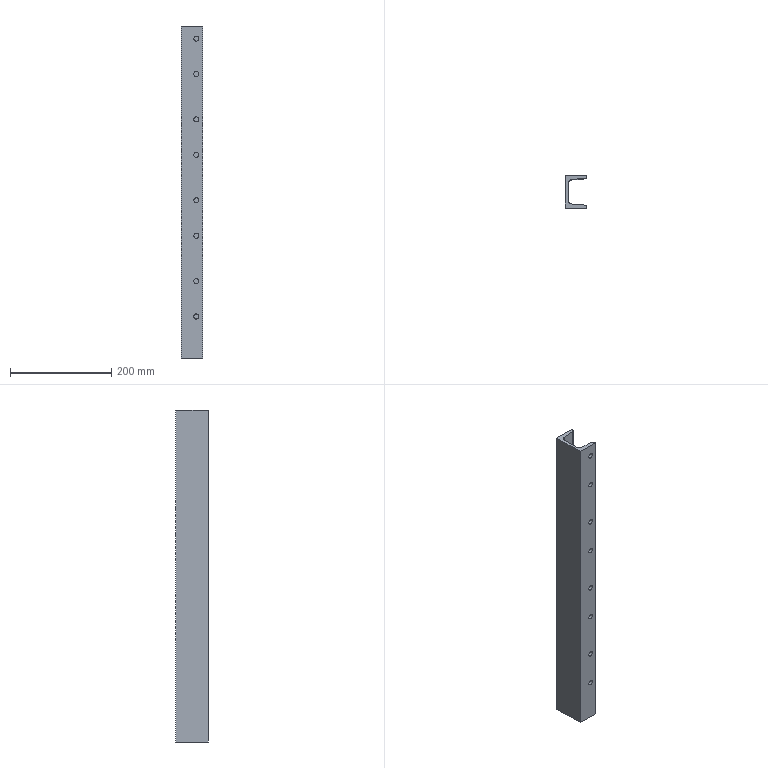Part | STEP file | DIN 1026-1 U 65 1785352674799 | 1 solid | 22 faces | box 42 x 65 x 657.157 mm | volume 589289 mm3 | cylinder 12 | plane 10 | commonest cylinder face diameters 10 x8 8 x2 15 x2
STEP:
#1=CARTESIAN_POINT('',(12.402,-24.312,657.157));
#2=VERTEX_POINT('',#1);
#3=CARTESIAN_POINT('',(38.319,-26.386,657.157));
#4=VERTEX_POINT('',#3);
#5=CARTESIAN_POINT('',(15.707,-24.577,657.157));
#6=DIRECTION('',(0.9968,-0.07975,0.));
#7=VECTOR('',#6,10.);
#8=LINE('',#5,#7);
#9=EDGE_CURVE('',#2,#4,#8,.T.);
#10=ORIENTED_EDGE('',*,*,#9,.F.);
#11=CARTESIAN_POINT('',(5.5,-16.836,657.157));
#12=VERTEX_POINT('',#11);
#13=CARTESIAN_POINT('',(13.,-16.836,657.157));
#14=DIRECTION('',(0.,0.,1.));
#15=DIRECTION('',(-1.,0.,0.));
#16=AXIS2_PLACEMENT_3D('',#13,#14,#15);
#17=CIRCLE('',#16,7.5);
#18=EDGE_CURVE('',#12,#2,#17,.T.);
#19=ORIENTED_EDGE('',*,*,#18,.F.);
#20=CARTESIAN_POINT('',(5.5,16.836,657.157));
#21=VERTEX_POINT('',#20);
#22=CARTESIAN_POINT('',(5.5,0.,657.157));
#23=DIRECTION('',(0.,-1.,0.));
#24=VECTOR('',#23,10.);
#25=LINE('',#22,#24);
#26=EDGE_CURVE('',#21,#12,#25,.T.);
#27=ORIENTED_EDGE('',*,*,#26,.F.);
#28=CARTESIAN_POINT('',(12.402,24.312,657.157));
#29=VERTEX_POINT('',#28);
#30=CARTESIAN_POINT('',(13.,16.836,657.157));
#31=DIRECTION('',(0.,0.,1.));
#32=DIRECTION('',(-0.07975,0.9968,0.));
#33=AXIS2_PLACEMENT_3D('',#30,#31,#32);
#34=CIRCLE('',#33,7.5);
#35=EDGE_CURVE('',#29,#21,#34,.T.);
#36=ORIENTED_EDGE('',*,*,#35,.F.);
#37=CARTESIAN_POINT('',(38.319,26.386,657.157));
#38=VERTEX_POINT('',#37);
#39=CARTESIAN_POINT('',(28.666,25.613,657.157));
#40=DIRECTION('',(-0.9968,-0.07975,0.));
#41=VECTOR('',#40,10.);
#42=LINE('',#39,#41);
#43=EDGE_CURVE('',#38,#29,#42,.T.);
#44=ORIENTED_EDGE('',*,*,#43,.F.);
#45=CARTESIAN_POINT('',(42.,30.373,657.157));
#46=VERTEX_POINT('',#45);
#47=CARTESIAN_POINT('',(38.,30.373,657.157));
#48=DIRECTION('',(0.,0.,-1.));
#49=DIRECTION('',(-0.07975,0.9968,0.));
#50=AXIS2_PLACEMENT_3D('',#47,#48,#49);
#51=CIRCLE('',#50,4.);
#52=EDGE_CURVE('',#46,#38,#51,.T.);
#53=ORIENTED_EDGE('',*,*,#52,.F.);
#54=CARTESIAN_POINT('',(42.,32.5,657.157));
#55=VERTEX_POINT('',#54);
#56=CARTESIAN_POINT('',(42.,16.25,657.157));
#57=DIRECTION('',(0.,-1.,0.));
#58=VECTOR('',#57,10.);
#59=LINE('',#56,#58);
#60=EDGE_CURVE('',#55,#46,#59,.T.);
#61=ORIENTED_EDGE('',*,*,#60,.F.);
#62=CARTESIAN_POINT('',(0.,32.5,657.157));
#63=VERTEX_POINT('',#62);
#64=CARTESIAN_POINT('',(10.5,32.5,657.157));
#65=DIRECTION('',(1.,0.,0.));
#66=VECTOR('',#65,10.);
#67=LINE('',#64,#66);
#68=EDGE_CURVE('',#63,#55,#67,.T.);
#69=ORIENTED_EDGE('',*,*,#68,.F.);
#70=CARTESIAN_POINT('',(0.,-32.5,657.157));
#71=VERTEX_POINT('',#70);
#72=CARTESIAN_POINT('',(0.,0.,657.157));
#73=DIRECTION('',(0.,1.,0.));
#74=VECTOR('',#73,10.);
#75=LINE('',#72,#74);
#76=EDGE_CURVE('',#71,#63,#75,.T.);
#77=ORIENTED_EDGE('',*,*,#76,.F.);
#78=CARTESIAN_POINT('',(42.,-32.5,657.157));
#79=VERTEX_POINT('',#78);
#80=CARTESIAN_POINT('',(31.5,-32.5,657.157));
#81=DIRECTION('',(-1.,0.,0.));
#82=VECTOR('',#81,10.);
#83=LINE('',#80,#82);
#84=EDGE_CURVE('',#79,#71,#83,.T.);
#85=ORIENTED_EDGE('',*,*,#84,.F.);
#86=CARTESIAN_POINT('',(42.,-30.373,657.157));
#87=VERTEX_POINT('',#86);
#88=CARTESIAN_POINT('',(42.,-15.186,657.157));
#89=DIRECTION('',(0.,-1.,0.));
#90=VECTOR('',#89,10.);
#91=LINE('',#88,#90);
#92=EDGE_CURVE('',#87,#79,#91,.T.);
#93=ORIENTED_EDGE('',*,*,#92,.F.);
#94=CARTESIAN_POINT('',(38.,-30.373,657.157));
#95=DIRECTION('',(0.,0.,-1.));
#96=DIRECTION('',(-1.,0.,0.));
#97=AXIS2_PLACEMENT_3D('',#94,#95,#96);
#98=CIRCLE('',#97,4.);
#99=EDGE_CURVE('',#4,#87,#98,.T.);
#100=ORIENTED_EDGE('',*,*,#99,.F.);
#101=EDGE_LOOP('',(#10,#19,#27,#36,#44,#53,#61,#69,#77,#85,#93,#100));
#102=FACE_OUTER_BOUND('',#101,.T.);
#103=CARTESIAN_POINT('',(21.,0.,657.157));
#104=DIRECTION('',(0.,0.,1.));
#105=DIRECTION('',(-1.,0.,0.));
#106=AXIS2_PLACEMENT_3D('',#103,#104,#105);
#107=PLANE('',#106);
#108=ADVANCED_FACE('',(#102),#107,.T.);
#109=ORIENTED_EDGE('',*,*,#52,.T.);
#110=CARTESIAN_POINT('',(38.319,26.386,0.));
#111=VERTEX_POINT('',#110);
#112=CARTESIAN_POINT('',(38.319,26.386,0.));
#113=DIRECTION('',(0.,0.,1.));
#114=VECTOR('',#113,10.);
#115=LINE('',#112,#114);
#116=EDGE_CURVE('',#111,#38,#115,.T.);
#117=ORIENTED_EDGE('',*,*,#116,.F.);
#118=CARTESIAN_POINT('',(42.,30.373,0.));
#119=VERTEX_POINT('',#118);
#120=CARTESIAN_POINT('',(38.,30.373,0.));
#121=DIRECTION('',(0.,0.,-1.));
#122=DIRECTION('',(-0.07975,0.9968,0.));
#123=AXIS2_PLACEMENT_3D('',#120,#121,#122);
#124=CIRCLE('',#123,4.);
#125=EDGE_CURVE('',#119,#111,#124,.T.);
#126=ORIENTED_EDGE('',*,*,#125,.F.);
#127=CARTESIAN_POINT('',(42.,30.373,0.));
#128=DIRECTION('',(0.,0.,1.));
#129=VECTOR('',#128,10.);
#130=LINE('',#127,#129);
#131=EDGE_CURVE('',#119,#46,#130,.T.);
#132=ORIENTED_EDGE('',*,*,#131,.T.);
#133=EDGE_LOOP('',(#109,#117,#126,#132));
#134=FACE_OUTER_BOUND('',#133,.T.);
#135=CARTESIAN_POINT('',(38.,30.373,0.));
#136=DIRECTION('',(0.,0.,1.));
#137=DIRECTION('',(-0.07975,0.9968,0.));
#138=AXIS2_PLACEMENT_3D('',#135,#136,#137);
#139=CYLINDRICAL_SURFACE('',#138,4.);
#140=ADVANCED_FACE('',(#134),#139,.T.);
#141=ORIENTED_EDGE('',*,*,#43,.T.);
#142=CARTESIAN_POINT('',(12.402,24.312,0.));
#143=VERTEX_POINT('',#142);
#144=CARTESIAN_POINT('',(12.402,24.312,0.));
#145=DIRECTION('',(0.,0.,1.));
#146=VECTOR('',#145,10.);
#147=LINE('',#144,#146);
#148=EDGE_CURVE('',#143,#29,#147,.T.);
#149=ORIENTED_EDGE('',*,*,#148,.F.);
#150=CARTESIAN_POINT('',(28.666,25.613,0.));
#151=DIRECTION('',(-0.9968,-0.07975,0.));
#152=VECTOR('',#151,10.);
#153=LINE('',#150,#152);
#154=EDGE_CURVE('',#111,#143,#153,.T.);
#155=ORIENTED_EDGE('',*,*,#154,.F.);
#156=ORIENTED_EDGE('',*,*,#116,.T.);
#157=EDGE_LOOP('',(#141,#149,#155,#156));
#158=FACE_OUTER_BOUND('',#157,.T.);
#159=CARTESIAN_POINT('',(38.319,26.386,0.));
#160=DIRECTION('',(0.07975,-0.9968,0.));
#161=DIRECTION('',(0.,0.,-1.));
#162=AXIS2_PLACEMENT_3D('',#159,#160,#161);
#163=PLANE('',#162);
#164=ADVANCED_FACE('',(#158),#163,.T.);
#165=ORIENTED_EDGE('',*,*,#35,.T.);
#166=CARTESIAN_POINT('',(5.5,16.836,0.));
#167=VERTEX_POINT('',#166);
#168=CARTESIAN_POINT('',(5.5,16.836,0.));
#169=DIRECTION('',(0.,0.,1.));
#170=VECTOR('',#169,10.);
#171=LINE('',#168,#170);
#172=EDGE_CURVE('',#167,#21,#171,.T.);
#173=ORIENTED_EDGE('',*,*,#172,.F.);
#174=CARTESIAN_POINT('',(13.,16.836,0.));
#175=DIRECTION('',(0.,0.,1.));
#176=DIRECTION('',(-0.07975,0.9968,0.));
#177=AXIS2_PLACEMENT_3D('',#174,#175,#176);
#178=CIRCLE('',#177,7.5);
#179=EDGE_CURVE('',#143,#167,#178,.T.);
#180=ORIENTED_EDGE('',*,*,#179,.F.);
#181=ORIENTED_EDGE('',*,*,#148,.T.);
#182=EDGE_LOOP('',(#165,#173,#180,#181));
#183=FACE_OUTER_BOUND('',#182,.T.);
#184=CARTESIAN_POINT('',(13.,16.836,0.));
#185=DIRECTION('',(0.,0.,1.));
#186=DIRECTION('',(-0.07975,0.9968,0.));
#187=AXIS2_PLACEMENT_3D('',#184,#185,#186);
#188=CYLINDRICAL_SURFACE('',#187,7.5);
#189=ADVANCED_FACE('',(#183),#188,.F.);
#190=ORIENTED_EDGE('',*,*,#26,.T.);
#191=CARTESIAN_POINT('',(5.5,-16.836,0.));
#192=VERTEX_POINT('',#191);
#193=CARTESIAN_POINT('',(5.5,-16.836,0.));
#194=DIRECTION('',(0.,0.,1.));
#195=VECTOR('',#194,10.);
#196=LINE('',#193,#195);
#197=EDGE_CURVE('',#192,#12,#196,.T.);
#198=ORIENTED_EDGE('',*,*,#197,.F.);
#199=CARTESIAN_POINT('',(5.5,0.,0.));
#200=DIRECTION('',(0.,-1.,0.));
#201=VECTOR('',#200,10.);
#202=LINE('',#199,#201);
#203=EDGE_CURVE('',#167,#192,#202,.T.);
#204=ORIENTED_EDGE('',*,*,#203,.F.);
#205=ORIENTED_EDGE('',*,*,#172,.T.);
#206=EDGE_LOOP('',(#190,#198,#204,#205));
#207=FACE_OUTER_BOUND('',#206,.T.);
#208=CARTESIAN_POINT('',(5.5,0.,0.));
#209=DIRECTION('',(1.,0.,0.));
#210=DIRECTION('',(0.,0.,-1.));
#211=AXIS2_PLACEMENT_3D('',#208,#209,#210);
#212=PLANE('',#211);
#213=ADVANCED_FACE('',(#207),#212,.T.);
#214=ORIENTED_EDGE('',*,*,#18,.T.);
#215=CARTESIAN_POINT('',(12.402,-24.312,0.));
#216=VERTEX_POINT('',#215);
#217=CARTESIAN_POINT('',(12.402,-24.312,0.));
#218=DIRECTION('',(0.,0.,1.));
#219=VECTOR('',#218,10.);
#220=LINE('',#217,#219);
#221=EDGE_CURVE('',#216,#2,#220,.T.);
#222=ORIENTED_EDGE('',*,*,#221,.F.);
#223=CARTESIAN_POINT('',(13.,-16.836,0.));
#224=DIRECTION('',(0.,0.,1.));
#225=DIRECTION('',(-1.,0.,0.));
#226=AXIS2_PLACEMENT_3D('',#223,#224,#225);
#227=CIRCLE('',#226,7.5);
#228=EDGE_CURVE('',#192,#216,#227,.T.);
#229=ORIENTED_EDGE('',*,*,#228,.F.);
#230=ORIENTED_EDGE('',*,*,#197,.T.);
#231=EDGE_LOOP('',(#214,#222,#229,#230));
#232=FACE_OUTER_BOUND('',#231,.T.);
#233=CARTESIAN_POINT('',(13.,-16.836,0.));
#234=DIRECTION('',(0.,0.,1.));
#235=DIRECTION('',(-1.,0.,0.));
#236=AXIS2_PLACEMENT_3D('',#233,#234,#235);
#237=CYLINDRICAL_SURFACE('',#236,7.5);
#238=ADVANCED_FACE('',(#232),#237,.F.);
#239=ORIENTED_EDGE('',*,*,#9,.T.);
#240=CARTESIAN_POINT('',(38.319,-26.386,0.));
#241=VERTEX_POINT('',#240);
#242=CARTESIAN_POINT('',(38.319,-26.386,0.));
#243=DIRECTION('',(0.,0.,1.));
#244=VECTOR('',#243,10.);
#245=LINE('',#242,#244);
#246=EDGE_CURVE('',#241,#4,#245,.T.);
#247=ORIENTED_EDGE('',*,*,#246,.F.);
#248=CARTESIAN_POINT('',(15.707,-24.577,0.));
#249=DIRECTION('',(0.9968,-0.07975,0.));
#250=VECTOR('',#249,10.);
#251=LINE('',#248,#250);
#252=EDGE_CURVE('',#216,#241,#251,.T.);
#253=ORIENTED_EDGE('',*,*,#252,.F.);
#254=ORIENTED_EDGE('',*,*,#221,.T.);
#255=EDGE_LOOP('',(#239,#247,#253,#254));
#256=FACE_OUTER_BOUND('',#255,.T.);
#257=CARTESIAN_POINT('',(34.5,-26.08,632.157));
#258=VERTEX_POINT('',#257);
#259=CARTESIAN_POINT('',(29.5,-25.68,632.157));
#260=DIRECTION('',(-0.07975,-0.9968,0.));
#261=DIRECTION('',(-0.9968,0.07975,0.));
#262=AXIS2_PLACEMENT_3D('',#259,#260,#261);
#263=ELLIPSE('',#262,5.016,5.);
#264=EDGE_CURVE('',#258,#258,#263,.T.);
#265=ORIENTED_EDGE('',*,*,#264,.T.);
#266=EDGE_LOOP('',(#265));
#267=FACE_BOUND('',#266,.T.);
#268=CARTESIAN_POINT('',(34.5,-26.08,562.157));
#269=VERTEX_POINT('',#268);
#270=CARTESIAN_POINT('',(29.5,-25.68,562.157));
#271=DIRECTION('',(-0.07975,-0.9968,0.));
#272=DIRECTION('',(-0.9968,0.07975,0.));
#273=AXIS2_PLACEMENT_3D('',#270,#271,#272);
#274=ELLIPSE('',#273,5.016,5.);
#275=EDGE_CURVE('',#269,#269,#274,.T.);
#276=ORIENTED_EDGE('',*,*,#275,.T.);
#277=EDGE_LOOP('',(#276));
#278=FACE_BOUND('',#277,.T.);
#279=CARTESIAN_POINT('',(34.5,-26.08,472.157));
#280=VERTEX_POINT('',#279);
#281=CARTESIAN_POINT('',(29.5,-25.68,472.157));
#282=DIRECTION('',(-0.07975,-0.9968,0.));
#283=DIRECTION('',(-0.9968,0.07975,0.));
#284=AXIS2_PLACEMENT_3D('',#281,#282,#283);
#285=ELLIPSE('',#284,5.016,5.);
#286=EDGE_CURVE('',#280,#280,#285,.T.);
#287=ORIENTED_EDGE('',*,*,#286,.T.);
#288=EDGE_LOOP('',(#287));
#289=FACE_BOUND('',#288,.T.);
#290=CARTESIAN_POINT('',(34.5,-26.08,402.157));
#291=VERTEX_POINT('',#290);
#292=CARTESIAN_POINT('',(29.5,-25.68,402.157));
#293=DIRECTION('',(-0.07975,-0.9968,0.));
#294=DIRECTION('',(-0.9968,0.07975,0.));
#295=AXIS2_PLACEMENT_3D('',#292,#293,#294);
#296=ELLIPSE('',#295,5.016,5.);
#297=EDGE_CURVE('',#291,#291,#296,.T.);
#298=ORIENTED_EDGE('',*,*,#297,.T.);
#299=EDGE_LOOP('',(#298));
#300=FACE_BOUND('',#299,.T.);
#301=CARTESIAN_POINT('',(34.5,-26.08,312.157));
#302=VERTEX_POINT('',#301);
#303=CARTESIAN_POINT('',(29.5,-25.68,312.157));
#304=DIRECTION('',(-0.07975,-0.9968,0.));
#305=DIRECTION('',(-0.9968,0.07975,0.));
#306=AXIS2_PLACEMENT_3D('',#303,#304,#305);
#307=ELLIPSE('',#306,5.016,5.);
#308=EDGE_CURVE('',#302,#302,#307,.T.);
#309=ORIENTED_EDGE('',*,*,#308,.T.);
#310=EDGE_LOOP('',(#309));
#311=FACE_BOUND('',#310,.T.);
#312=CARTESIAN_POINT('',(34.5,-26.08,242.157));
#313=VERTEX_POINT('',#312);
#314=CARTESIAN_POINT('',(29.5,-25.68,242.157));
#315=DIRECTION('',(-0.07975,-0.9968,0.));
#316=DIRECTION('',(-0.9968,0.07975,0.));
#317=AXIS2_PLACEMENT_3D('',#314,#315,#316);
#318=ELLIPSE('',#317,5.016,5.);
#319=EDGE_CURVE('',#313,#313,#318,.T.);
#320=ORIENTED_EDGE('',*,*,#319,.T.);
#321=EDGE_LOOP('',(#320));
#322=FACE_BOUND('',#321,.T.);
#323=CARTESIAN_POINT('',(34.5,-26.08,152.157));
#324=VERTEX_POINT('',#323);
#325=CARTESIAN_POINT('',(29.5,-25.68,152.157));
#326=DIRECTION('',(-0.07975,-0.9968,0.));
#327=DIRECTION('',(-0.9968,0.07975,0.));
#328=AXIS2_PLACEMENT_3D('',#325,#326,#327);
#329=ELLIPSE('',#328,5.016,5.);
#330=EDGE_CURVE('',#324,#324,#329,.T.);
#331=ORIENTED_EDGE('',*,*,#330,.T.);
#332=EDGE_LOOP('',(#331));
#333=FACE_BOUND('',#332,.T.);
#334=CARTESIAN_POINT('',(34.5,-26.08,82.157));
#335=VERTEX_POINT('',#334);
#336=CARTESIAN_POINT('',(29.5,-25.68,82.157));
#337=DIRECTION('',(-0.07975,-0.9968,0.));
#338=DIRECTION('',(-0.9968,0.07975,0.));
#339=AXIS2_PLACEMENT_3D('',#336,#337,#338);
#340=ELLIPSE('',#339,5.016,5.);
#341=EDGE_CURVE('',#335,#335,#340,.T.);
#342=ORIENTED_EDGE('',*,*,#341,.T.);
#343=EDGE_LOOP('',(#342));
#344=FACE_BOUND('',#343,.T.);
#345=CARTESIAN_POINT('',(12.402,-24.312,0.));
#346=DIRECTION('',(0.07975,0.9968,0.));
#347=DIRECTION('',(0.,0.,1.));
#348=AXIS2_PLACEMENT_3D('',#345,#346,#347);
#349=PLANE('',#348);
#350=ADVANCED_FACE('',(#256,#267,#278,#289,#300,#311,#322,#333,#344),#349,.T.);
#351=CARTESIAN_POINT('',(34.5,-32.5,82.157));
#352=VERTEX_POINT('',#351);
#353=CARTESIAN_POINT('',(29.5,-32.5,82.157));
#354=DIRECTION('',(0.,1.,0.));
#355=DIRECTION('',(-1.,0.,0.));
#356=AXIS2_PLACEMENT_3D('',#353,#354,#355);
#357=CIRCLE('',#356,5.);
#358=EDGE_CURVE('',#352,#352,#357,.T.);
#359=ORIENTED_EDGE('',*,*,#358,.F.);
#360=CARTESIAN_POINT('',(34.5,-32.5,82.157));
#361=DIRECTION('',(0.,1.,0.));
#362=VECTOR('',#361,5.);
#363=LINE('',#360,#362);
#364=EDGE_CURVE('',#352,#335,#363,.T.);
#365=ORIENTED_EDGE('',*,*,#364,.T.);
#366=ORIENTED_EDGE('',*,*,#341,.F.);
#367=ORIENTED_EDGE('',*,*,#364,.F.);
#368=EDGE_LOOP('',(#359,#365,#366,#367));
#369=FACE_OUTER_BOUND('',#368,.T.);
#370=CARTESIAN_POINT('',(29.5,-32.5,82.157));
#371=DIRECTION('',(0.,1.,0.));
#372=DIRECTION('',(-1.,0.,0.));
#373=AXIS2_PLACEMENT_3D('',#370,#371,#372);
#374=CYLINDRICAL_SURFACE('',#373,5.);
#375=ADVANCED_FACE('',(#369),#374,.F.);
#376=CARTESIAN_POINT('',(34.5,-32.5,152.157));
#377=VERTEX_POINT('',#376);
#378=CARTESIAN_POINT('',(29.5,-32.5,152.157));
#379=DIRECTION('',(0.,1.,0.));
#380=DIRECTION('',(-1.,0.,0.));
#381=AXIS2_PLACEMENT_3D('',#378,#379,#380);
#382=CIRCLE('',#381,5.);
#383=EDGE_CURVE('',#377,#377,#382,.T.);
#384=ORIENTED_EDGE('',*,*,#383,.F.);
#385=CARTESIAN_POINT('',(34.5,-32.5,152.157));
#386=DIRECTION('',(0.,1.,0.));
#387=VECTOR('',#386,5.);
#388=LINE('',#385,#387);
#389=EDGE_CURVE('',#377,#324,#388,.T.);
#390=ORIENTED_EDGE('',*,*,#389,.T.);
#391=ORIENTED_EDGE('',*,*,#330,.F.);
#392=ORIENTED_EDGE('',*,*,#389,.F.);
#393=EDGE_LOOP('',(#384,#390,#391,#392));
#394=FACE_OUTER_BOUND('',#393,.T.);
#395=CARTESIAN_POINT('',(29.5,-32.5,152.157));
#396=DIRECTION('',(0.,1.,0.));
#397=DIRECTION('',(-1.,0.,0.));
#398=AXIS2_PLACEMENT_3D('',#395,#396,#397);
#399=CYLINDRICAL_SURFACE('',#398,5.);
#400=ADVANCED_FACE('',(#394),#399,.F.);
#401=CARTESIAN_POINT('',(34.5,-32.5,242.157));
#402=VERTEX_POINT('',#401);
#403=CARTESIAN_POINT('',(29.5,-32.5,242.157));
#404=DIRECTION('',(0.,1.,0.));
#405=DIRECTION('',(-1.,0.,0.));
#406=AXIS2_PLACEMENT_3D('',#403,#404,#405);
#407=CIRCLE('',#406,5.);
#408=EDGE_CURVE('',#402,#402,#407,.T.);
#409=ORIENTED_EDGE('',*,*,#408,.F.);
#410=CARTESIAN_POINT('',(34.5,-32.5,242.157));
#411=DIRECTION('',(0.,1.,0.));
#412=VECTOR('',#411,5.);
#413=LINE('',#410,#412);
#414=EDGE_CURVE('',#402,#313,#413,.T.);
#415=ORIENTED_EDGE('',*,*,#414,.T.);
#416=ORIENTED_EDGE('',*,*,#319,.F.);
#417=ORIENTED_EDGE('',*,*,#414,.F.);
#418=EDGE_LOOP('',(#409,#415,#416,#417));
#419=FACE_OUTER_BOUND('',#418,.T.);
#420=CARTESIAN_POINT('',(29.5,-32.5,242.157));
#421=DIRECTION('',(0.,1.,0.));
#422=DIRECTION('',(-1.,0.,0.));
#423=AXIS2_PLACEMENT_3D('',#420,#421,#422);
#424=CYLINDRICAL_SURFACE('',#423,5.);
#425=ADVANCED_FACE('',(#419),#424,.F.);
#426=CARTESIAN_POINT('',(34.5,-32.5,312.157));
#427=VERTEX_POINT('',#426);
#428=CARTESIAN_POINT('',(29.5,-32.5,312.157));
#429=DIRECTION('',(0.,1.,0.));
#430=DIRECTION('',(-1.,0.,0.));
#431=AXIS2_PLACEMENT_3D('',#428,#429,#430);
#432=CIRCLE('',#431,5.);
#433=EDGE_CURVE('',#427,#427,#432,.T.);
#434=ORIENTED_EDGE('',*,*,#433,.F.);
#435=CARTESIAN_POINT('',(34.5,-32.5,312.157));
#436=DIRECTION('',(0.,1.,0.));
#437=VECTOR('',#436,5.);
#438=LINE('',#435,#437);
#439=EDGE_CURVE('',#427,#302,#438,.T.);
#440=ORIENTED_EDGE('',*,*,#439,.T.);
#441=ORIENTED_EDGE('',*,*,#308,.F.);
#442=ORIENTED_EDGE('',*,*,#439,.F.);
#443=EDGE_LOOP('',(#434,#440,#441,#442));
#444=FACE_OUTER_BOUND('',#443,.T.);
#445=CARTESIAN_POINT('',(29.5,-32.5,312.157));
#446=DIRECTION('',(0.,1.,0.));
#447=DIRECTION('',(-1.,0.,0.));
#448=AXIS2_PLACEMENT_3D('',#445,#446,#447);
#449=CYLINDRICAL_SURFACE('',#448,5.);
#450=ADVANCED_FACE('',(#444),#449,.F.);
#451=CARTESIAN_POINT('',(34.5,-32.5,402.157));
#452=VERTEX_POINT('',#451);
#453=CARTESIAN_POINT('',(29.5,-32.5,402.157));
#454=DIRECTION('',(0.,1.,0.));
#455=DIRECTION('',(-1.,0.,0.));
#456=AXIS2_PLACEMENT_3D('',#453,#454,#455);
#457=CIRCLE('',#456,5.);
#458=EDGE_CURVE('',#452,#452,#457,.T.);
#459=ORIENTED_EDGE('',*,*,#458,.F.);
#460=CARTESIAN_POINT('',(34.5,-32.5,402.157));
#461=DIRECTION('',(0.,1.,0.));
#462=VECTOR('',#461,5.);
#463=LINE('',#460,#462);
#464=EDGE_CURVE('',#452,#291,#463,.T.);
#465=ORIENTED_EDGE('',*,*,#464,.T.);
#466=ORIENTED_EDGE('',*,*,#297,.F.);
#467=ORIENTED_EDGE('',*,*,#464,.F.);
#468=EDGE_LOOP('',(#459,#465,#466,#467));
#469=FACE_OUTER_BOUND('',#468,.T.);
#470=CARTESIAN_POINT('',(29.5,-32.5,402.157));
#471=DIRECTION('',(0.,1.,0.));
#472=DIRECTION('',(-1.,0.,0.));
#473=AXIS2_PLACEMENT_3D('',#470,#471,#472);
#474=CYLINDRICAL_SURFACE('',#473,5.);
#475=ADVANCED_FACE('',(#469),#474,.F.);
#476=CARTESIAN_POINT('',(34.5,-32.5,472.157));
#477=VERTEX_POINT('',#476);
#478=CARTESIAN_POINT('',(29.5,-32.5,472.157));
#479=DIRECTION('',(0.,1.,0.));
#480=DIRECTION('',(-1.,0.,0.));
#481=AXIS2_PLACEMENT_3D('',#478,#479,#480);
#482=CIRCLE('',#481,5.);
#483=EDGE_CURVE('',#477,#477,#482,.T.);
#484=ORIENTED_EDGE('',*,*,#483,.F.);
#485=CARTESIAN_POINT('',(34.5,-32.5,472.157));
#486=DIRECTION('',(0.,1.,0.));
#487=VECTOR('',#486,5.);
#488=LINE('',#485,#487);
#489=EDGE_CURVE('',#477,#280,#488,.T.);
#490=ORIENTED_EDGE('',*,*,#489,.T.);
#491=ORIENTED_EDGE('',*,*,#286,.F.);
#492=ORIENTED_EDGE('',*,*,#489,.F.);
#493=EDGE_LOOP('',(#484,#490,#491,#492));
#494=FACE_OUTER_BOUND('',#493,.T.);
#495=CARTESIAN_POINT('',(29.5,-32.5,472.157));
#496=DIRECTION('',(0.,1.,0.));
#497=DIRECTION('',(-1.,0.,0.));
#498=AXIS2_PLACEMENT_3D('',#495,#496,#497);
#499=CYLINDRICAL_SURFACE('',#498,5.);
#500=ADVANCED_FACE('',(#494),#499,.F.);
#501=CARTESIAN_POINT('',(34.5,-32.5,562.157));
#502=VERTEX_POINT('',#501);
#503=CARTESIAN_POINT('',(29.5,-32.5,562.157));
#504=DIRECTION('',(0.,1.,0.));
#505=DIRECTION('',(-1.,0.,0.));
#506=AXIS2_PLACEMENT_3D('',#503,#504,#505);
#507=CIRCLE('',#506,5.);
#508=EDGE_CURVE('',#502,#502,#507,.T.);
#509=ORIENTED_EDGE('',*,*,#508,.F.);
#510=CARTESIAN_POINT('',(34.5,-32.5,562.157));
#511=DIRECTION('',(0.,1.,0.));
#512=VECTOR('',#511,5.);
#513=LINE('',#510,#512);
#514=EDGE_CURVE('',#502,#269,#513,.T.);
#515=ORIENTED_EDGE('',*,*,#514,.T.);
#516=ORIENTED_EDGE('',*,*,#275,.F.);
#517=ORIENTED_EDGE('',*,*,#514,.F.);
#518=EDGE_LOOP('',(#509,#515,#516,#517));
#519=FACE_OUTER_BOUND('',#518,.T.);
#520=CARTESIAN_POINT('',(29.5,-32.5,562.157));
#521=DIRECTION('',(0.,1.,0.));
#522=DIRECTION('',(-1.,0.,0.));
#523=AXIS2_PLACEMENT_3D('',#520,#521,#522);
#524=CYLINDRICAL_SURFACE('',#523,5.);
#525=ADVANCED_FACE('',(#519),#524,.F.);
#526=CARTESIAN_POINT('',(34.5,-32.5,632.157));
#527=VERTEX_POINT('',#526);
#528=CARTESIAN_POINT('',(29.5,-32.5,632.157));
#529=DIRECTION('',(0.,1.,0.));
#530=DIRECTION('',(-1.,0.,0.));
#531=AXIS2_PLACEMENT_3D('',#528,#529,#530);
#532=CIRCLE('',#531,5.);
#533=EDGE_CURVE('',#527,#527,#532,.T.);
#534=ORIENTED_EDGE('',*,*,#533,.F.);
#535=CARTESIAN_POINT('',(34.5,-32.5,632.157));
#536=DIRECTION('',(0.,1.,0.));
#537=VECTOR('',#536,5.);
#538=LINE('',#535,#537);
#539=EDGE_CURVE('',#527,#258,#538,.T.);
#540=ORIENTED_EDGE('',*,*,#539,.T.);
#541=ORIENTED_EDGE('',*,*,#264,.F.);
#542=ORIENTED_EDGE('',*,*,#539,.F.);
#543=EDGE_LOOP('',(#534,#540,#541,#542));
#544=FACE_OUTER_BOUND('',#543,.T.);
#545=CARTESIAN_POINT('',(29.5,-32.5,632.157));
#546=DIRECTION('',(0.,1.,0.));
#547=DIRECTION('',(-1.,0.,0.));
#548=AXIS2_PLACEMENT_3D('',#545,#546,#547);
#549=CYLINDRICAL_SURFACE('',#548,5.);
#550=ADVANCED_FACE('',(#544),#549,.F.);
#551=ORIENTED_EDGE('',*,*,#99,.T.);
#552=CARTESIAN_POINT('',(42.,-30.373,0.));
#553=VERTEX_POINT('',#552);
#554=CARTESIAN_POINT('',(42.,-30.373,0.));
#555=DIRECTION('',(0.,0.,1.));
#556=VECTOR('',#555,10.);
#557=LINE('',#554,#556);
#558=EDGE_CURVE('',#553,#87,#557,.T.);
#559=ORIENTED_EDGE('',*,*,#558,.F.);
#560=CARTESIAN_POINT('',(38.,-30.373,0.));
#561=DIRECTION('',(0.,0.,-1.));
#562=DIRECTION('',(-1.,0.,0.));
#563=AXIS2_PLACEMENT_3D('',#560,#561,#562);
#564=CIRCLE('',#563,4.);
#565=EDGE_CURVE('',#241,#553,#564,.T.);
#566=ORIENTED_EDGE('',*,*,#565,.F.);
#567=ORIENTED_EDGE('',*,*,#246,.T.);
#568=EDGE_LOOP('',(#551,#559,#566,#567));
#569=FACE_OUTER_BOUND('',#568,.T.);
#570=CARTESIAN_POINT('',(38.,-30.373,0.));
#571=DIRECTION('',(0.,0.,1.));
#572=DIRECTION('',(-1.,0.,0.));
#573=AXIS2_PLACEMENT_3D('',#570,#571,#572);
#574=CYLINDRICAL_SURFACE('',#573,4.);
#575=ADVANCED_FACE('',(#569),#574,.T.);
#576=ORIENTED_EDGE('',*,*,#92,.T.);
#577=CARTESIAN_POINT('',(42.,-32.5,0.));
#578=VERTEX_POINT('',#577);
#579=CARTESIAN_POINT('',(42.,-32.5,0.));
#580=DIRECTION('',(0.,0.,1.));
#581=VECTOR('',#580,10.);
#582=LINE('',#579,#581);
#583=EDGE_CURVE('',#578,#79,#582,.T.);
#584=ORIENTED_EDGE('',*,*,#583,.F.);
#585=CARTESIAN_POINT('',(42.,-15.186,0.));
#586=DIRECTION('',(0.,-1.,0.));
#587=VECTOR('',#586,10.);
#588=LINE('',#585,#587);
#589=EDGE_CURVE('',#553,#578,#588,.T.);
#590=ORIENTED_EDGE('',*,*,#589,.F.);
#591=ORIENTED_EDGE('',*,*,#558,.T.);
#592=EDGE_LOOP('',(#576,#584,#590,#591));
#593=FACE_OUTER_BOUND('',#592,.T.);
#594=CARTESIAN_POINT('',(42.,-30.373,0.));
#595=DIRECTION('',(1.,0.,0.));
#596=DIRECTION('',(0.,0.,-1.));
#597=AXIS2_PLACEMENT_3D('',#594,#595,#596);
#598=PLANE('',#597);
#599=ADVANCED_FACE('',(#593),#598,.T.);
#600=ORIENTED_EDGE('',*,*,#84,.T.);
#601=CARTESIAN_POINT('',(0.,-32.5,0.));
#602=VERTEX_POINT('',#601);
#603=CARTESIAN_POINT('',(0.,-32.5,0.));
#604=DIRECTION('',(0.,0.,1.));
#605=VECTOR('',#604,10.);
#606=LINE('',#603,#605);
#607=EDGE_CURVE('',#602,#71,#606,.T.);
#608=ORIENTED_EDGE('',*,*,#607,.F.);
#609=CARTESIAN_POINT('',(31.5,-32.5,0.));
#610=DIRECTION('',(-1.,0.,0.));
#611=VECTOR('',#610,10.);
#612=LINE('',#609,#611);
#613=EDGE_CURVE('',#578,#602,#612,.T.);
#614=ORIENTED_EDGE('',*,*,#613,.F.);
#615=ORIENTED_EDGE('',*,*,#583,.T.);
#616=EDGE_LOOP('',(#600,#608,#614,#615));
#617=FACE_OUTER_BOUND('',#616,.T.);
#618=ORIENTED_EDGE('',*,*,#358,.T.);
#619=EDGE_LOOP('',(#618));
#620=FACE_BOUND('',#619,.T.);
#621=ORIENTED_EDGE('',*,*,#383,.T.);
#622=EDGE_LOOP('',(#621));
#623=FACE_BOUND('',#622,.T.);
#624=ORIENTED_EDGE('',*,*,#408,.T.);
#625=EDGE_LOOP('',(#624));
#626=FACE_BOUND('',#625,.T.);
#627=ORIENTED_EDGE('',*,*,#433,.T.);
#628=EDGE_LOOP('',(#627));
#629=FACE_BOUND('',#628,.T.);
#630=ORIENTED_EDGE('',*,*,#458,.T.);
#631=EDGE_LOOP('',(#630));
#632=FACE_BOUND('',#631,.T.);
#633=ORIENTED_EDGE('',*,*,#483,.T.);
#634=EDGE_LOOP('',(#633));
#635=FACE_BOUND('',#634,.T.);
#636=ORIENTED_EDGE('',*,*,#508,.T.);
#637=EDGE_LOOP('',(#636));
#638=FACE_BOUND('',#637,.T.);
#639=ORIENTED_EDGE('',*,*,#533,.T.);
#640=EDGE_LOOP('',(#639));
#641=FACE_BOUND('',#640,.T.);
#642=CARTESIAN_POINT('',(42.,-32.5,0.));
#643=DIRECTION('',(0.,-1.,0.));
#644=DIRECTION('',(0.,0.,-1.));
#645=AXIS2_PLACEMENT_3D('',#642,#643,#644);
#646=PLANE('',#645);
#647=ADVANCED_FACE('',(#617,#620,#623,#626,#629,#632,#635,#638,#641),#646,.T.);
#648=ORIENTED_EDGE('',*,*,#76,.T.);
#649=CARTESIAN_POINT('',(0.,32.5,0.));
#650=VERTEX_POINT('',#649);
#651=CARTESIAN_POINT('',(0.,32.5,0.));
#652=DIRECTION('',(0.,0.,1.));
#653=VECTOR('',#652,10.);
#654=LINE('',#651,#653);
#655=EDGE_CURVE('',#650,#63,#654,.T.);
#656=ORIENTED_EDGE('',*,*,#655,.F.);
#657=CARTESIAN_POINT('',(0.,0.,0.));
#658=DIRECTION('',(0.,1.,0.));
#659=VECTOR('',#658,10.);
#660=LINE('',#657,#659);
#661=EDGE_CURVE('',#602,#650,#660,.T.);
#662=ORIENTED_EDGE('',*,*,#661,.F.);
#663=ORIENTED_EDGE('',*,*,#607,.T.);
#664=EDGE_LOOP('',(#648,#656,#662,#663));
#665=FACE_OUTER_BOUND('',#664,.T.);
#666=CARTESIAN_POINT('',(0.,0.,0.));
#667=DIRECTION('',(-1.,0.,0.));
#668=DIRECTION('',(0.,0.,1.));
#669=AXIS2_PLACEMENT_3D('',#666,#667,#668);
#670=PLANE('',#669);
#671=ADVANCED_FACE('',(#665),#670,.T.);
#672=ORIENTED_EDGE('',*,*,#68,.T.);
#673=CARTESIAN_POINT('',(42.,32.5,0.));
#674=VERTEX_POINT('',#673);
#675=CARTESIAN_POINT('',(42.,32.5,0.));
#676=DIRECTION('',(0.,0.,1.));
#677=VECTOR('',#676,10.);
#678=LINE('',#675,#677);
#679=EDGE_CURVE('',#674,#55,#678,.T.);
#680=ORIENTED_EDGE('',*,*,#679,.F.);
#681=CARTESIAN_POINT('',(10.5,32.5,0.));
#682=DIRECTION('',(1.,0.,0.));
#683=VECTOR('',#682,10.);
#684=LINE('',#681,#683);
#685=EDGE_CURVE('',#650,#674,#684,.T.);
#686=ORIENTED_EDGE('',*,*,#685,.F.);
#687=ORIENTED_EDGE('',*,*,#655,.T.);
#688=EDGE_LOOP('',(#672,#680,#686,#687));
#689=FACE_OUTER_BOUND('',#688,.T.);
#690=CARTESIAN_POINT('',(0.,32.5,0.));
#691=DIRECTION('',(0.,1.,0.));
#692=DIRECTION('',(0.,0.,1.));
#693=AXIS2_PLACEMENT_3D('',#690,#691,#692);
#694=PLANE('',#693);
#695=ADVANCED_FACE('',(#689),#694,.T.);
#696=ORIENTED_EDGE('',*,*,#60,.T.);
#697=ORIENTED_EDGE('',*,*,#131,.F.);
#698=CARTESIAN_POINT('',(42.,16.25,0.));
#699=DIRECTION('',(0.,-1.,0.));
#700=VECTOR('',#699,10.);
#701=LINE('',#698,#700);
#702=EDGE_CURVE('',#674,#119,#701,.T.);
#703=ORIENTED_EDGE('',*,*,#702,.F.);
#704=ORIENTED_EDGE('',*,*,#679,.T.);
#705=EDGE_LOOP('',(#696,#697,#703,#704));
#706=FACE_OUTER_BOUND('',#705,.T.);
#707=CARTESIAN_POINT('',(42.,32.5,0.));
#708=DIRECTION('',(1.,0.,0.));
#709=DIRECTION('',(0.,0.,-1.));
#710=AXIS2_PLACEMENT_3D('',#707,#708,#709);
#711=PLANE('',#710);
#712=ADVANCED_FACE('',(#706),#711,.T.);
#713=ORIENTED_EDGE('',*,*,#685,.T.);
#714=ORIENTED_EDGE('',*,*,#702,.T.);
#715=ORIENTED_EDGE('',*,*,#125,.T.);
#716=ORIENTED_EDGE('',*,*,#154,.T.);
#717=ORIENTED_EDGE('',*,*,#179,.T.);
#718=ORIENTED_EDGE('',*,*,#203,.T.);
#719=ORIENTED_EDGE('',*,*,#228,.T.);
#720=ORIENTED_EDGE('',*,*,#252,.T.);
#721=ORIENTED_EDGE('',*,*,#565,.T.);
#722=ORIENTED_EDGE('',*,*,#589,.T.);
#723=ORIENTED_EDGE('',*,*,#613,.T.);
#724=ORIENTED_EDGE('',*,*,#661,.T.);
#725=EDGE_LOOP('',(#713,#714,#715,#716,#717,#718,#719,#720,#721,#722,#723,#724));
#726=FACE_OUTER_BOUND('',#725,.T.);
#727=CARTESIAN_POINT('',(21.,0.,0.));
#728=DIRECTION('',(0.,0.,1.));
#729=DIRECTION('',(1.,0.,0.));
#730=AXIS2_PLACEMENT_3D('',#727,#728,#729);
#731=PLANE('',#730);
#732=ADVANCED_FACE('',(#726),#731,.F.);
#733=CLOSED_SHELL('',(#108,#140,#164,#189,#213,#238,#350,#375,#400,#425,#450,#475,#500,#525,#550,#575,#599,#647,#671,#695,#712,#732));
#734=MANIFOLD_SOLID_BREP('',#733);
#735=(LENGTH_UNIT()NAMED_UNIT(*)SI_UNIT(.MILLI.,.METRE.));
#736=UNCERTAINTY_MEASURE_WITH_UNIT(LENGTH_MEASURE(0.01),#735,'','');
#737=(NAMED_UNIT(*)PLANE_ANGLE_UNIT()SI_UNIT($,.RADIAN.));
#738=(NAMED_UNIT(*)SI_UNIT($,.STERADIAN.)SOLID_ANGLE_UNIT());
#739=(GEOMETRIC_REPRESENTATION_CONTEXT(3)GLOBAL_UNCERTAINTY_ASSIGNED_CONTEXT((#736))GLOBAL_UNIT_ASSIGNED_CONTEXT((#735,#737,#738))REPRESENTATION_CONTEXT('',''));
#740=ADVANCED_BREP_SHAPE_REPRESENTATION('',(#734),#739);